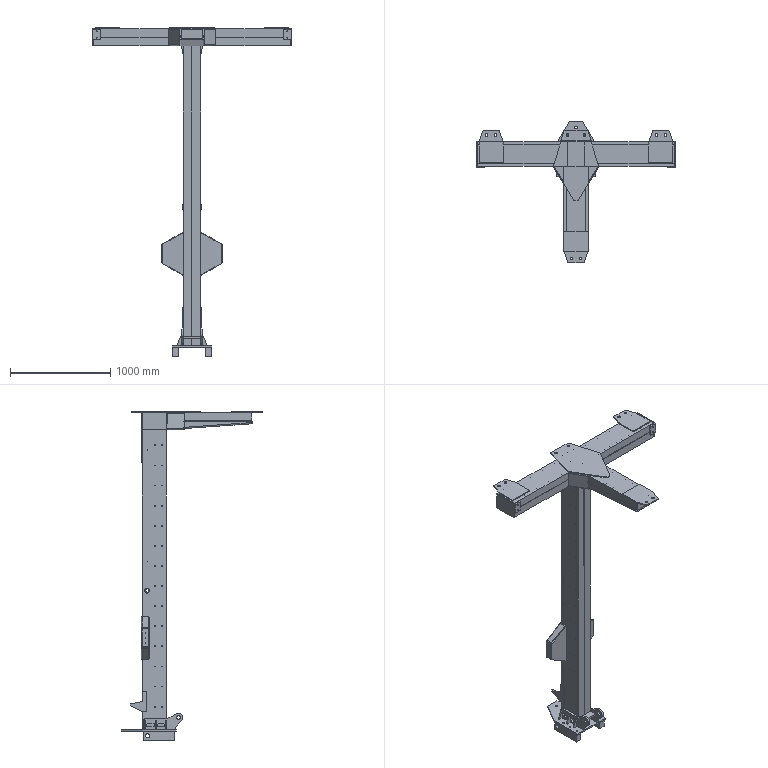Part | SolidWorks | features CompositeCurve 1 | 40 solids | 668 faces | box 1980 x 1410 x 3270 mm | volume 66085382 mm3 | plane 340 | cylinder 308 | cone 16 | sphere 4 | commonest cylinder face diameters 8.5 x112 6.8 x32 20 x20 10.2 x18 13 x18 17 x16